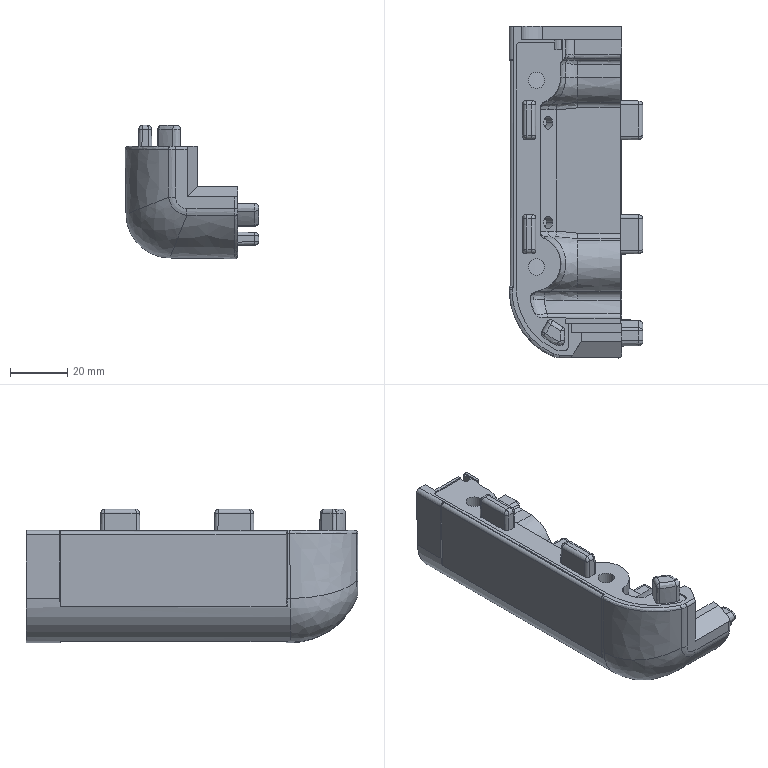Part | SolidWorks | features BaseBody 1, ICE 1 | 1 solid | 481 faces | box 46.838 x 116.267 x 46.838 mm | volume 58227 mm3 | cylinder 176 | spline 162 | plane 131 | torus 10 | cone 2 | commonest cylinder face diameters 0.6 x28 2.9 x22 2.4 x21 1.5 x20 2.5 x16 2 x11